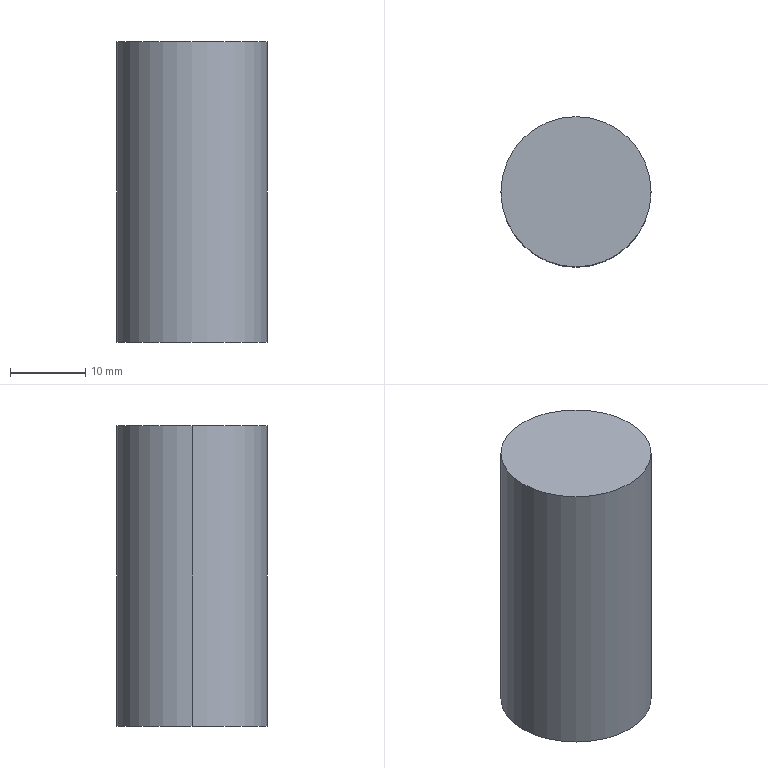Part | SolidWorks | features Extrusion 1 | 1 solid | 4 faces | box 20 x 20 x 40 mm | volume 12566 mm3 | cylinder 2 | plane 2 | commonest cylinder face diameters 20 x2
STEP:
#1=CARTESIAN_POINT('',(10.,0.,20.));
#2=VERTEX_POINT('',#1);
#3=CARTESIAN_POINT('',(-10.,0.,20.));
#4=VERTEX_POINT('',#3);
#5=CARTESIAN_POINT('',(0.,0.,20.));
#6=DIRECTION('',(0.,0.,1.));
#7=DIRECTION('',(1.,0.,0.));
#8=AXIS2_PLACEMENT_3D('',#5,#6,#7);
#9=CIRCLE('',#8,10.);
#10=EDGE_CURVE('',#2,#4,#9,.T.);
#11=ORIENTED_EDGE('',*,*,#10,.F.);
#12=CARTESIAN_POINT('',(10.,0.,-20.));
#13=VERTEX_POINT('',#12);
#14=CARTESIAN_POINT('',(10.,0.,20.));
#15=DIRECTION('',(0.,0.,-1.));
#16=VECTOR('',#15,1000.);
#17=LINE('',#14,#16);
#18=EDGE_CURVE('',#2,#13,#17,.T.);
#19=ORIENTED_EDGE('',*,*,#18,.T.);
#20=CARTESIAN_POINT('',(-10.,0.,-20.));
#21=VERTEX_POINT('',#20);
#22=CARTESIAN_POINT('',(0.,0.,-20.));
#23=DIRECTION('',(0.,0.,1.));
#24=DIRECTION('',(1.,0.,0.));
#25=AXIS2_PLACEMENT_3D('',#22,#23,#24);
#26=CIRCLE('',#25,10.);
#27=EDGE_CURVE('',#13,#21,#26,.T.);
#28=ORIENTED_EDGE('',*,*,#27,.T.);
#29=CARTESIAN_POINT('',(-10.,0.,20.));
#30=DIRECTION('',(0.,0.,-1.));
#31=VECTOR('',#30,1000.);
#32=LINE('',#29,#31);
#33=EDGE_CURVE('',#4,#21,#32,.T.);
#34=ORIENTED_EDGE('',*,*,#33,.F.);
#35=EDGE_LOOP('',(#11,#19,#28,#34));
#36=FACE_OUTER_BOUND('',#35,.T.);
#37=CARTESIAN_POINT('',(0.,0.,20.));
#38=DIRECTION('',(0.,0.,-1.));
#39=DIRECTION('',(-1.,0.,0.));
#40=AXIS2_PLACEMENT_3D('',#37,#38,#39);
#41=CYLINDRICAL_SURFACE('',#40,10.);
#42=ADVANCED_FACE('',(#36),#41,.T.);
#43=ORIENTED_EDGE('',*,*,#18,.F.);
#44=CARTESIAN_POINT('',(0.,0.,20.));
#45=DIRECTION('',(0.,0.,1.));
#46=DIRECTION('',(1.,0.,0.));
#47=AXIS2_PLACEMENT_3D('',#44,#45,#46);
#48=CIRCLE('',#47,10.);
#49=EDGE_CURVE('',#4,#2,#48,.T.);
#50=ORIENTED_EDGE('',*,*,#49,.F.);
#51=ORIENTED_EDGE('',*,*,#33,.T.);
#52=CARTESIAN_POINT('',(0.,0.,-20.));
#53=DIRECTION('',(0.,0.,1.));
#54=DIRECTION('',(1.,0.,0.));
#55=AXIS2_PLACEMENT_3D('',#52,#53,#54);
#56=CIRCLE('',#55,10.);
#57=EDGE_CURVE('',#21,#13,#56,.T.);
#58=ORIENTED_EDGE('',*,*,#57,.T.);
#59=EDGE_LOOP('',(#43,#50,#51,#58));
#60=FACE_OUTER_BOUND('',#59,.T.);
#61=CARTESIAN_POINT('',(0.,0.,20.));
#62=DIRECTION('',(0.,0.,-1.));
#63=DIRECTION('',(-1.,0.,0.));
#64=AXIS2_PLACEMENT_3D('',#61,#62,#63);
#65=CYLINDRICAL_SURFACE('',#64,10.);
#66=ADVANCED_FACE('',(#60),#65,.T.);
#67=ORIENTED_EDGE('',*,*,#49,.T.);
#68=ORIENTED_EDGE('',*,*,#10,.T.);
#69=EDGE_LOOP('',(#67,#68));
#70=FACE_OUTER_BOUND('',#69,.T.);
#71=CARTESIAN_POINT('',(0.,0.,20.));
#72=DIRECTION('',(0.,0.,1.));
#73=DIRECTION('',(1.,0.,0.));
#74=AXIS2_PLACEMENT_3D('',#71,#72,#73);
#75=PLANE('',#74);
#76=ADVANCED_FACE('',(#70),#75,.T.);
#77=ORIENTED_EDGE('',*,*,#57,.F.);
#78=ORIENTED_EDGE('',*,*,#27,.F.);
#79=EDGE_LOOP('',(#77,#78));
#80=FACE_OUTER_BOUND('',#79,.T.);
#81=CARTESIAN_POINT('',(0.,0.,-20.));
#82=DIRECTION('',(0.,0.,1.));
#83=DIRECTION('',(1.,0.,0.));
#84=AXIS2_PLACEMENT_3D('',#81,#82,#83);
#85=PLANE('',#84);
#86=ADVANCED_FACE('',(#80),#85,.F.);
#87=CLOSED_SHELL('',(#42,#66,#76,#86));
#88=MANIFOLD_SOLID_BREP('',#87);
#89=CARTESIAN_POINT('',(0.,0.,0.));
#90=DIRECTION('',(0.,0.,1.));
#91=DIRECTION('',(1.,0.,0.));
#92=AXIS2_PLACEMENT_3D('',#89,#90,#91);
#93=(LENGTH_UNIT()NAMED_UNIT(*)SI_UNIT(.MILLI.,.METRE.));
#94=UNCERTAINTY_MEASURE_WITH_UNIT(LENGTH_MEASURE(0.00001),#93,'','');
#95=(NAMED_UNIT(*)PLANE_ANGLE_UNIT()SI_UNIT($,.RADIAN.));
#96=(NAMED_UNIT(*)SI_UNIT($,.STERADIAN.)SOLID_ANGLE_UNIT());
#97=(GEOMETRIC_REPRESENTATION_CONTEXT(3)GLOBAL_UNCERTAINTY_ASSIGNED_CONTEXT((#94))GLOBAL_UNIT_ASSIGNED_CONTEXT((#93,#95,#96))REPRESENTATION_CONTEXT('',''));
#98=ADVANCED_BREP_SHAPE_REPRESENTATION('',(#88,#92),#97);